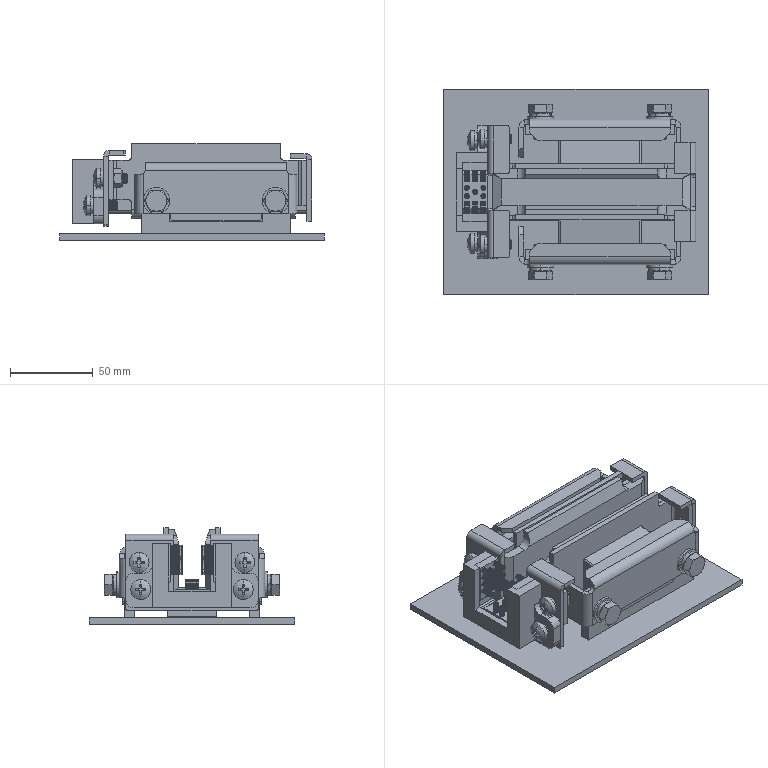Part | SolidWorks | features BaseBody 39, ICE 1, MoveCopyBody 1 | 39 solids | 6314 faces | volume 358287 mm3 | cylinder 3780 | plane 2014 | cone 512 | sphere 8 | commonest cylinder face diameters 0.3 x2684 0.4 x648 6 x204 4 x32 10 x30 4.917 x28